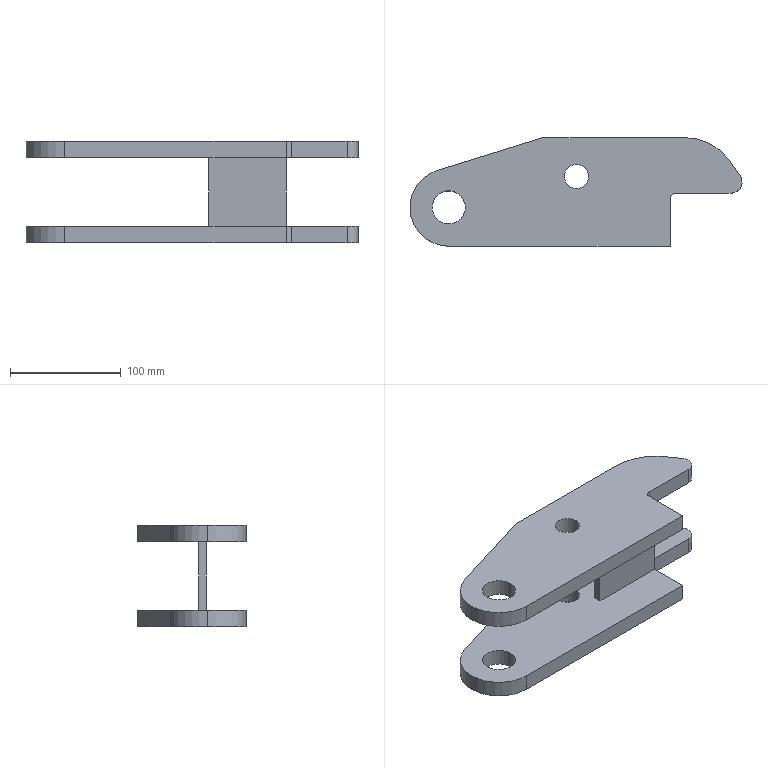Part | SolidWorks | features ICE 2, Extrusion 1, Fillet 1, LPattern 1 | 1 solid | 36 faces | box 300 x 98 x 92 mm | volume 689780 mm3 | cylinder 18 | plane 18 | commonest cylinder face diameters 22 x4 30 x4 70 x4 10 x2 20 x2 100 x2
STEP:
#1=CARTESIAN_POINT('',(-91.605,144.,-1575.828));
#2=VERTEX_POINT('',#1);
#3=CARTESIAN_POINT('',(-69.605,144.,-1575.828));
#4=VERTEX_POINT('',#3);
#5=CARTESIAN_POINT('',(-80.605,144.,-1575.828));
#6=DIRECTION('',(0.,0.,1.));
#7=DIRECTION('',(1.,0.,0.));
#8=AXIS2_PLACEMENT_3D('',#5,#6,#7);
#9=CIRCLE('',#8,11.);
#10=EDGE_CURVE('',#2,#4,#9,.T.);
#11=ORIENTED_EDGE('',*,*,#10,.T.);
#12=CARTESIAN_POINT('',(-69.605,144.,-1590.828));
#13=VERTEX_POINT('',#12);
#14=CARTESIAN_POINT('',(-69.605,144.,-1408.828));
#15=DIRECTION('',(0.,0.,-1.));
#16=VECTOR('',#15,1000.);
#17=LINE('',#14,#16);
#18=EDGE_CURVE('',#4,#13,#17,.T.);
#19=ORIENTED_EDGE('',*,*,#18,.T.);
#20=CARTESIAN_POINT('',(-91.605,144.,-1590.828));
#21=VERTEX_POINT('',#20);
#22=CARTESIAN_POINT('',(-80.605,144.,-1590.828));
#23=DIRECTION('',(0.,0.,1.));
#24=DIRECTION('',(1.,0.,0.));
#25=AXIS2_PLACEMENT_3D('',#22,#23,#24);
#26=CIRCLE('',#25,11.);
#27=EDGE_CURVE('',#21,#13,#26,.T.);
#28=ORIENTED_EDGE('',*,*,#27,.F.);
#29=CARTESIAN_POINT('',(-91.605,144.,-1408.828));
#30=DIRECTION('',(0.,0.,-1.));
#31=VECTOR('',#30,1000.);
#32=LINE('',#29,#31);
#33=EDGE_CURVE('',#2,#21,#32,.T.);
#34=ORIENTED_EDGE('',*,*,#33,.F.);
#35=EDGE_LOOP('',(#11,#19,#28,#34));
#36=FACE_OUTER_BOUND('',#35,.T.);
#37=CARTESIAN_POINT('',(-80.605,144.,-1408.828));
#38=DIRECTION('',(0.,0.,-1.));
#39=DIRECTION('',(-1.,0.,0.));
#40=AXIS2_PLACEMENT_3D('',#37,#38,#39);
#41=CYLINDRICAL_SURFACE('',#40,11.);
#42=ADVANCED_FACE('',(#36),#41,.F.);
#43=CARTESIAN_POINT('',(-91.605,144.,-1498.828));
#44=VERTEX_POINT('',#43);
#45=CARTESIAN_POINT('',(-69.605,144.,-1498.828));
#46=VERTEX_POINT('',#45);
#47=CARTESIAN_POINT('',(-80.605,144.,-1498.828));
#48=DIRECTION('',(0.,0.,1.));
#49=DIRECTION('',(1.,0.,0.));
#50=AXIS2_PLACEMENT_3D('',#47,#48,#49);
#51=CIRCLE('',#50,11.);
#52=EDGE_CURVE('',#44,#46,#51,.T.);
#53=ORIENTED_EDGE('',*,*,#52,.T.);
#54=CARTESIAN_POINT('',(-69.605,144.,-1513.828));
#55=VERTEX_POINT('',#54);
#56=CARTESIAN_POINT('',(-69.605,144.,-1408.828));
#57=DIRECTION('',(0.,0.,-1.));
#58=VECTOR('',#57,1000.);
#59=LINE('',#56,#58);
#60=EDGE_CURVE('',#46,#55,#59,.T.);
#61=ORIENTED_EDGE('',*,*,#60,.T.);
#62=CARTESIAN_POINT('',(-91.605,144.,-1513.828));
#63=VERTEX_POINT('',#62);
#64=CARTESIAN_POINT('',(-80.605,144.,-1513.828));
#65=DIRECTION('',(0.,0.,1.));
#66=DIRECTION('',(1.,0.,0.));
#67=AXIS2_PLACEMENT_3D('',#64,#65,#66);
#68=CIRCLE('',#67,11.);
#69=EDGE_CURVE('',#63,#55,#68,.T.);
#70=ORIENTED_EDGE('',*,*,#69,.F.);
#71=CARTESIAN_POINT('',(-91.605,144.,-1408.828));
#72=DIRECTION('',(0.,0.,-1.));
#73=VECTOR('',#72,1000.);
#74=LINE('',#71,#73);
#75=EDGE_CURVE('',#44,#63,#74,.T.);
#76=ORIENTED_EDGE('',*,*,#75,.F.);
#77=EDGE_LOOP('',(#53,#61,#70,#76));
#78=FACE_OUTER_BOUND('',#77,.T.);
#79=CARTESIAN_POINT('',(-80.605,144.,-1408.828));
#80=DIRECTION('',(0.,0.,-1.));
#81=DIRECTION('',(-1.,0.,0.));
#82=AXIS2_PLACEMENT_3D('',#79,#80,#81);
#83=CYLINDRICAL_SURFACE('',#82,11.);
#84=ADVANCED_FACE('',(#78),#83,.F.);
#85=CARTESIAN_POINT('',(-211.,116.,-1498.828));
#86=VERTEX_POINT('',#85);
#87=CARTESIAN_POINT('',(-181.,116.,-1498.828));
#88=VERTEX_POINT('',#87);
#89=CARTESIAN_POINT('',(-196.,116.,-1498.828));
#90=DIRECTION('',(0.,0.,1.));
#91=DIRECTION('',(1.,0.,0.));
#92=AXIS2_PLACEMENT_3D('',#89,#90,#91);
#93=CIRCLE('',#92,15.);
#94=EDGE_CURVE('',#86,#88,#93,.T.);
#95=ORIENTED_EDGE('',*,*,#94,.T.);
#96=CARTESIAN_POINT('',(-181.,116.,-1513.828));
#97=VERTEX_POINT('',#96);
#98=CARTESIAN_POINT('',(-181.,116.,-1498.828));
#99=DIRECTION('',(0.,0.,-1.));
#100=VECTOR('',#99,1000.);
#101=LINE('',#98,#100);
#102=EDGE_CURVE('',#88,#97,#101,.T.);
#103=ORIENTED_EDGE('',*,*,#102,.T.);
#104=CARTESIAN_POINT('',(-211.,116.,-1513.828));
#105=VERTEX_POINT('',#104);
#106=CARTESIAN_POINT('',(-196.,116.,-1513.828));
#107=DIRECTION('',(0.,0.,1.));
#108=DIRECTION('',(1.,0.,0.));
#109=AXIS2_PLACEMENT_3D('',#106,#107,#108);
#110=CIRCLE('',#109,15.);
#111=EDGE_CURVE('',#105,#97,#110,.T.);
#112=ORIENTED_EDGE('',*,*,#111,.F.);
#113=CARTESIAN_POINT('',(-211.,116.,-1498.828));
#114=DIRECTION('',(0.,0.,-1.));
#115=VECTOR('',#114,1000.);
#116=LINE('',#113,#115);
#117=EDGE_CURVE('',#86,#105,#116,.T.);
#118=ORIENTED_EDGE('',*,*,#117,.F.);
#119=EDGE_LOOP('',(#95,#103,#112,#118));
#120=FACE_OUTER_BOUND('',#119,.T.);
#121=CARTESIAN_POINT('',(-196.,116.,-1498.828));
#122=DIRECTION('',(0.,0.,-1.));
#123=DIRECTION('',(-1.,0.,0.));
#124=AXIS2_PLACEMENT_3D('',#121,#122,#123);
#125=CYLINDRICAL_SURFACE('',#124,15.);
#126=ADVANCED_FACE('',(#120),#125,.F.);
#127=CARTESIAN_POINT('',(-231.,116.,-1498.828));
#128=VERTEX_POINT('',#127);
#129=CARTESIAN_POINT('',(-196.,81.,-1498.828));
#130=VERTEX_POINT('',#129);
#131=CARTESIAN_POINT('',(-196.,116.,-1498.828));
#132=DIRECTION('',(0.,0.,1.));
#133=DIRECTION('',(1.,0.,0.));
#134=AXIS2_PLACEMENT_3D('',#131,#132,#133);
#135=CIRCLE('',#134,35.);
#136=EDGE_CURVE('',#128,#130,#135,.T.);
#137=ORIENTED_EDGE('',*,*,#136,.F.);
#138=CARTESIAN_POINT('',(-231.,116.,-1513.828));
#139=VERTEX_POINT('',#138);
#140=CARTESIAN_POINT('',(-231.,116.,-1498.828));
#141=DIRECTION('',(0.,0.,-1.));
#142=VECTOR('',#141,1000.);
#143=LINE('',#140,#142);
#144=EDGE_CURVE('',#128,#139,#143,.T.);
#145=ORIENTED_EDGE('',*,*,#144,.T.);
#146=CARTESIAN_POINT('',(-196.,81.,-1513.828));
#147=VERTEX_POINT('',#146);
#148=CARTESIAN_POINT('',(-196.,116.,-1513.828));
#149=DIRECTION('',(0.,0.,1.));
#150=DIRECTION('',(1.,0.,0.));
#151=AXIS2_PLACEMENT_3D('',#148,#149,#150);
#152=CIRCLE('',#151,35.);
#153=EDGE_CURVE('',#139,#147,#152,.T.);
#154=ORIENTED_EDGE('',*,*,#153,.T.);
#155=CARTESIAN_POINT('',(-196.,81.,-1498.828));
#156=DIRECTION('',(0.,0.,-1.));
#157=VECTOR('',#156,1000.);
#158=LINE('',#155,#157);
#159=EDGE_CURVE('',#130,#147,#158,.T.);
#160=ORIENTED_EDGE('',*,*,#159,.F.);
#161=EDGE_LOOP('',(#137,#145,#154,#160));
#162=FACE_OUTER_BOUND('',#161,.T.);
#163=CARTESIAN_POINT('',(-196.,116.,-1498.828));
#164=DIRECTION('',(0.,0.,-1.));
#165=DIRECTION('',(-1.,0.,0.));
#166=AXIS2_PLACEMENT_3D('',#163,#164,#165);
#167=CYLINDRICAL_SURFACE('',#166,35.);
#168=ADVANCED_FACE('',(#162),#167,.T.);
#169=CARTESIAN_POINT('',(-211.,116.,-1575.828));
#170=VERTEX_POINT('',#169);
#171=CARTESIAN_POINT('',(-181.,116.,-1575.828));
#172=VERTEX_POINT('',#171);
#173=CARTESIAN_POINT('',(-196.,116.,-1575.828));
#174=DIRECTION('',(0.,0.,1.));
#175=DIRECTION('',(1.,0.,0.));
#176=AXIS2_PLACEMENT_3D('',#173,#174,#175);
#177=CIRCLE('',#176,15.);
#178=EDGE_CURVE('',#170,#172,#177,.T.);
#179=ORIENTED_EDGE('',*,*,#178,.T.);
#180=CARTESIAN_POINT('',(-181.,116.,-1590.828));
#181=VERTEX_POINT('',#180);
#182=CARTESIAN_POINT('',(-181.,116.,-1575.828));
#183=DIRECTION('',(0.,0.,-1.));
#184=VECTOR('',#183,1000.);
#185=LINE('',#182,#184);
#186=EDGE_CURVE('',#172,#181,#185,.T.);
#187=ORIENTED_EDGE('',*,*,#186,.T.);
#188=CARTESIAN_POINT('',(-211.,116.,-1590.828));
#189=VERTEX_POINT('',#188);
#190=CARTESIAN_POINT('',(-196.,116.,-1590.828));
#191=DIRECTION('',(0.,0.,1.));
#192=DIRECTION('',(1.,0.,0.));
#193=AXIS2_PLACEMENT_3D('',#190,#191,#192);
#194=CIRCLE('',#193,15.);
#195=EDGE_CURVE('',#189,#181,#194,.T.);
#196=ORIENTED_EDGE('',*,*,#195,.F.);
#197=CARTESIAN_POINT('',(-211.,116.,-1575.828));
#198=DIRECTION('',(0.,0.,-1.));
#199=VECTOR('',#198,1000.);
#200=LINE('',#197,#199);
#201=EDGE_CURVE('',#170,#189,#200,.T.);
#202=ORIENTED_EDGE('',*,*,#201,.F.);
#203=EDGE_LOOP('',(#179,#187,#196,#202));
#204=FACE_OUTER_BOUND('',#203,.T.);
#205=CARTESIAN_POINT('',(-196.,116.,-1575.828));
#206=DIRECTION('',(0.,0.,-1.));
#207=DIRECTION('',(-1.,0.,0.));
#208=AXIS2_PLACEMENT_3D('',#205,#206,#207);
#209=CYLINDRICAL_SURFACE('',#208,15.);
#210=ADVANCED_FACE('',(#204),#209,.F.);
#211=CARTESIAN_POINT('',(-231.,116.,-1575.828));
#212=VERTEX_POINT('',#211);
#213=CARTESIAN_POINT('',(-196.,81.,-1575.828));
#214=VERTEX_POINT('',#213);
#215=CARTESIAN_POINT('',(-196.,116.,-1575.828));
#216=DIRECTION('',(0.,0.,1.));
#217=DIRECTION('',(1.,0.,0.));
#218=AXIS2_PLACEMENT_3D('',#215,#216,#217);
#219=CIRCLE('',#218,35.);
#220=EDGE_CURVE('',#212,#214,#219,.T.);
#221=ORIENTED_EDGE('',*,*,#220,.F.);
#222=CARTESIAN_POINT('',(-231.,116.,-1590.828));
#223=VERTEX_POINT('',#222);
#224=CARTESIAN_POINT('',(-231.,116.,-1575.828));
#225=DIRECTION('',(0.,0.,-1.));
#226=VECTOR('',#225,1000.);
#227=LINE('',#224,#226);
#228=EDGE_CURVE('',#212,#223,#227,.T.);
#229=ORIENTED_EDGE('',*,*,#228,.T.);
#230=CARTESIAN_POINT('',(-196.,81.,-1590.828));
#231=VERTEX_POINT('',#230);
#232=CARTESIAN_POINT('',(-196.,116.,-1590.828));
#233=DIRECTION('',(0.,0.,1.));
#234=DIRECTION('',(1.,0.,0.));
#235=AXIS2_PLACEMENT_3D('',#232,#233,#234);
#236=CIRCLE('',#235,35.);
#237=EDGE_CURVE('',#223,#231,#236,.T.);
#238=ORIENTED_EDGE('',*,*,#237,.T.);
#239=CARTESIAN_POINT('',(-196.,81.,-1575.828));
#240=DIRECTION('',(0.,0.,-1.));
#241=VECTOR('',#240,1000.);
#242=LINE('',#239,#241);
#243=EDGE_CURVE('',#214,#231,#242,.T.);
#244=ORIENTED_EDGE('',*,*,#243,.F.);
#245=EDGE_LOOP('',(#221,#229,#238,#244));
#246=FACE_OUTER_BOUND('',#245,.T.);
#247=CARTESIAN_POINT('',(-196.,116.,-1575.828));
#248=DIRECTION('',(0.,0.,-1.));
#249=DIRECTION('',(-1.,0.,0.));
#250=AXIS2_PLACEMENT_3D('',#247,#248,#249);
#251=CYLINDRICAL_SURFACE('',#250,35.);
#252=ADVANCED_FACE('',(#246),#251,.T.);
#253=ORIENTED_EDGE('',*,*,#10,.F.);
#254=CARTESIAN_POINT('',(-80.605,144.,-1575.828));
#255=DIRECTION('',(0.,0.,1.));
#256=DIRECTION('',(1.,0.,0.));
#257=AXIS2_PLACEMENT_3D('',#254,#255,#256);
#258=CIRCLE('',#257,11.);
#259=EDGE_CURVE('',#4,#2,#258,.T.);
#260=ORIENTED_EDGE('',*,*,#259,.F.);
#261=EDGE_LOOP('',(#253,#260));
#262=FACE_BOUND('',#261,.T.);
#263=CARTESIAN_POINT('',(-66.,117.,-1575.828));
#264=VERTEX_POINT('',#263);
#265=CARTESIAN_POINT('',(4.,117.,-1575.828));
#266=VERTEX_POINT('',#265);
#267=CARTESIAN_POINT('',(-66.,117.,-1575.828));
#268=DIRECTION('',(1.,0.,0.));
#269=VECTOR('',#268,1000.);
#270=LINE('',#267,#269);
#271=EDGE_CURVE('',#264,#266,#270,.T.);
#272=ORIENTED_EDGE('',*,*,#271,.F.);
#273=CARTESIAN_POINT('',(-66.,124.,-1575.828));
#274=VERTEX_POINT('',#273);
#275=CARTESIAN_POINT('',(-66.,124.,-1575.828));
#276=DIRECTION('',(0.,-1.,0.));
#277=VECTOR('',#276,1000.);
#278=LINE('',#275,#277);
#279=EDGE_CURVE('',#274,#264,#278,.T.);
#280=ORIENTED_EDGE('',*,*,#279,.F.);
#281=CARTESIAN_POINT('',(4.,124.,-1575.828));
#282=VERTEX_POINT('',#281);
#283=CARTESIAN_POINT('',(-66.,124.,-1575.828));
#284=DIRECTION('',(1.,0.,0.));
#285=VECTOR('',#284,1000.);
#286=LINE('',#283,#285);
#287=EDGE_CURVE('',#274,#282,#286,.T.);
#288=ORIENTED_EDGE('',*,*,#287,.T.);
#289=CARTESIAN_POINT('',(9.,129.,-1575.828));
#290=VERTEX_POINT('',#289);
#291=CARTESIAN_POINT('',(9.,124.,-1575.828));
#292=DIRECTION('',(0.,0.,-1.));
#293=DIRECTION('',(1.,0.,0.));
#294=AXIS2_PLACEMENT_3D('',#291,#292,#293);
#295=CIRCLE('',#294,5.);
#296=EDGE_CURVE('',#282,#290,#295,.T.);
#297=ORIENTED_EDGE('',*,*,#296,.T.);
#298=CARTESIAN_POINT('',(59.,129.,-1575.828));
#299=VERTEX_POINT('',#298);
#300=CARTESIAN_POINT('',(59.,129.,-1575.828));
#301=DIRECTION('',(1.,0.,0.));
#302=VECTOR('',#301,1000.);
#303=LINE('',#300,#302);
#304=EDGE_CURVE('',#290,#299,#303,.T.);
#305=ORIENTED_EDGE('',*,*,#304,.T.);
#306=CARTESIAN_POINT('',(67.203,144.719,-1575.828));
#307=VERTEX_POINT('',#306);
#308=CARTESIAN_POINT('',(59.,139.,-1575.828));
#309=DIRECTION('',(0.,0.,1.));
#310=DIRECTION('',(1.,0.,0.));
#311=AXIS2_PLACEMENT_3D('',#308,#309,#310);
#312=CIRCLE('',#311,10.);
#313=EDGE_CURVE('',#299,#307,#312,.T.);
#314=ORIENTED_EDGE('',*,*,#313,.T.);
#315=CARTESIAN_POINT('',(58.224,157.597,-1575.828));
#316=VERTEX_POINT('',#315);
#317=CARTESIAN_POINT('',(58.224,157.597,-1575.828));
#318=DIRECTION('',(-0.5719,0.8203,0.));
#319=VECTOR('',#318,1000.);
#320=LINE('',#317,#319);
#321=EDGE_CURVE('',#307,#316,#320,.T.);
#322=ORIENTED_EDGE('',*,*,#321,.T.);
#323=CARTESIAN_POINT('',(17.209,179.,-1575.828));
#324=VERTEX_POINT('',#323);
#325=CARTESIAN_POINT('',(17.209,129.,-1575.828));
#326=DIRECTION('',(0.,0.,1.));
#327=DIRECTION('',(-1.,0.,0.));
#328=AXIS2_PLACEMENT_3D('',#325,#326,#327);
#329=CIRCLE('',#328,50.);
#330=EDGE_CURVE('',#316,#324,#329,.T.);
#331=ORIENTED_EDGE('',*,*,#330,.T.);
#332=CARTESIAN_POINT('',(-111.,179.,-1575.828));
#333=VERTEX_POINT('',#332);
#334=CARTESIAN_POINT('',(17.209,179.,-1575.828));
#335=DIRECTION('',(-1.,0.,0.));
#336=VECTOR('',#335,1000.);
#337=LINE('',#334,#336);
#338=EDGE_CURVE('',#324,#333,#337,.T.);
#339=ORIENTED_EDGE('',*,*,#338,.T.);
#340=CARTESIAN_POINT('',(-206.366,149.43,-1575.828));
#341=VERTEX_POINT('',#340);
#342=CARTESIAN_POINT('',(-111.,179.,-1575.828));
#343=DIRECTION('',(-0.9551,-0.2962,0.));
#344=VECTOR('',#343,1000.);
#345=LINE('',#342,#344);
#346=EDGE_CURVE('',#333,#341,#345,.T.);
#347=ORIENTED_EDGE('',*,*,#346,.T.);
#348=CARTESIAN_POINT('',(-196.,116.,-1575.828));
#349=DIRECTION('',(0.,0.,1.));
#350=DIRECTION('',(1.,0.,0.));
#351=AXIS2_PLACEMENT_3D('',#348,#349,#350);
#352=CIRCLE('',#351,35.);
#353=EDGE_CURVE('',#341,#212,#352,.T.);
#354=ORIENTED_EDGE('',*,*,#353,.T.);
#355=ORIENTED_EDGE('',*,*,#220,.T.);
#356=CARTESIAN_POINT('',(4.,81.,-1575.828));
#357=VERTEX_POINT('',#356);
#358=CARTESIAN_POINT('',(4.,81.,-1575.828));
#359=DIRECTION('',(1.,0.,0.));
#360=VECTOR('',#359,1000.);
#361=LINE('',#358,#360);
#362=EDGE_CURVE('',#214,#357,#361,.T.);
#363=ORIENTED_EDGE('',*,*,#362,.T.);
#364=CARTESIAN_POINT('',(4.,129.,-1575.828));
#365=DIRECTION('',(0.,1.,0.));
#366=VECTOR('',#365,1000.);
#367=LINE('',#364,#366);
#368=EDGE_CURVE('',#357,#266,#367,.T.);
#369=ORIENTED_EDGE('',*,*,#368,.T.);
#370=EDGE_LOOP('',(#272,#280,#288,#297,#305,#314,#322,#331,#339,#347,#354,#355,#363,#369));
#371=FACE_OUTER_BOUND('',#370,.T.);
#372=ORIENTED_EDGE('',*,*,#178,.F.);
#373=CARTESIAN_POINT('',(-196.,116.,-1575.828));
#374=DIRECTION('',(0.,0.,1.));
#375=DIRECTION('',(1.,0.,0.));
#376=AXIS2_PLACEMENT_3D('',#373,#374,#375);
#377=CIRCLE('',#376,15.);
#378=EDGE_CURVE('',#172,#170,#377,.T.);
#379=ORIENTED_EDGE('',*,*,#378,.F.);
#380=EDGE_LOOP('',(#372,#379));
#381=FACE_BOUND('',#380,.T.);
#382=CARTESIAN_POINT('',(-196.,116.,-1575.828));
#383=DIRECTION('',(0.,0.,1.));
#384=DIRECTION('',(1.,0.,0.));
#385=AXIS2_PLACEMENT_3D('',#382,#383,#384);
#386=PLANE('',#385);
#387=ADVANCED_FACE('',(#262,#371,#381),#386,.T.);
#388=ORIENTED_EDGE('',*,*,#27,.T.);
#389=CARTESIAN_POINT('',(-80.605,144.,-1590.828));
#390=DIRECTION('',(0.,0.,1.));
#391=DIRECTION('',(1.,0.,0.));
#392=AXIS2_PLACEMENT_3D('',#389,#390,#391);
#393=CIRCLE('',#392,11.);
#394=EDGE_CURVE('',#13,#21,#393,.T.);
#395=ORIENTED_EDGE('',*,*,#394,.T.);
#396=EDGE_LOOP('',(#388,#395));
#397=FACE_BOUND('',#396,.T.);
#398=CARTESIAN_POINT('',(4.,81.,-1590.828));
#399=VERTEX_POINT('',#398);
#400=CARTESIAN_POINT('',(4.,124.,-1590.828));
#401=VERTEX_POINT('',#400);
#402=CARTESIAN_POINT('',(4.,129.,-1590.828));
#403=DIRECTION('',(0.,1.,0.));
#404=VECTOR('',#403,1000.);
#405=LINE('',#402,#404);
#406=EDGE_CURVE('',#399,#401,#405,.T.);
#407=ORIENTED_EDGE('',*,*,#406,.F.);
#408=CARTESIAN_POINT('',(4.,81.,-1590.828));
#409=DIRECTION('',(1.,0.,0.));
#410=VECTOR('',#409,1000.);
#411=LINE('',#408,#410);
#412=EDGE_CURVE('',#231,#399,#411,.T.);
#413=ORIENTED_EDGE('',*,*,#412,.F.);
#414=ORIENTED_EDGE('',*,*,#237,.F.);
#415=CARTESIAN_POINT('',(-206.366,149.43,-1590.828));
#416=VERTEX_POINT('',#415);
#417=CARTESIAN_POINT('',(-196.,116.,-1590.828));
#418=DIRECTION('',(0.,0.,1.));
#419=DIRECTION('',(1.,0.,0.));
#420=AXIS2_PLACEMENT_3D('',#417,#418,#419);
#421=CIRCLE('',#420,35.);
#422=EDGE_CURVE('',#416,#223,#421,.T.);
#423=ORIENTED_EDGE('',*,*,#422,.F.);
#424=CARTESIAN_POINT('',(-111.,179.,-1590.828));
#425=VERTEX_POINT('',#424);
#426=CARTESIAN_POINT('',(-111.,179.,-1590.828));
#427=DIRECTION('',(-0.9551,-0.2962,0.));
#428=VECTOR('',#427,1000.);
#429=LINE('',#426,#428);
#430=EDGE_CURVE('',#425,#416,#429,.T.);
#431=ORIENTED_EDGE('',*,*,#430,.F.);
#432=CARTESIAN_POINT('',(17.209,179.,-1590.828));
#433=VERTEX_POINT('',#432);
#434=CARTESIAN_POINT('',(17.209,179.,-1590.828));
#435=DIRECTION('',(-1.,0.,0.));
#436=VECTOR('',#435,1000.);
#437=LINE('',#434,#436);
#438=EDGE_CURVE('',#433,#425,#437,.T.);
#439=ORIENTED_EDGE('',*,*,#438,.F.);
#440=CARTESIAN_POINT('',(58.224,157.597,-1590.828));
#441=VERTEX_POINT('',#440);
#442=CARTESIAN_POINT('',(17.209,129.,-1590.828));
#443=DIRECTION('',(0.,0.,1.));
#444=DIRECTION('',(-1.,0.,0.));
#445=AXIS2_PLACEMENT_3D('',#442,#443,#444);
#446=CIRCLE('',#445,50.);
#447=EDGE_CURVE('',#441,#433,#446,.T.);
#448=ORIENTED_EDGE('',*,*,#447,.F.);
#449=CARTESIAN_POINT('',(67.203,144.719,-1590.828));
#450=VERTEX_POINT('',#449);
#451=CARTESIAN_POINT('',(58.224,157.597,-1590.828));
#452=DIRECTION('',(-0.5719,0.8203,0.));
#453=VECTOR('',#452,1000.);
#454=LINE('',#451,#453);
#455=EDGE_CURVE('',#450,#441,#454,.T.);
#456=ORIENTED_EDGE('',*,*,#455,.F.);
#457=CARTESIAN_POINT('',(59.,129.,-1590.828));
#458=VERTEX_POINT('',#457);
#459=CARTESIAN_POINT('',(59.,139.,-1590.828));
#460=DIRECTION('',(0.,0.,1.));
#461=DIRECTION('',(1.,0.,0.));
#462=AXIS2_PLACEMENT_3D('',#459,#460,#461);
#463=CIRCLE('',#462,10.);
#464=EDGE_CURVE('',#458,#450,#463,.T.);
#465=ORIENTED_EDGE('',*,*,#464,.F.);
#466=CARTESIAN_POINT('',(9.,129.,-1590.828));
#467=VERTEX_POINT('',#466);
#468=CARTESIAN_POINT('',(59.,129.,-1590.828));
#469=DIRECTION('',(1.,0.,0.));
#470=VECTOR('',#469,1000.);
#471=LINE('',#468,#470);
#472=EDGE_CURVE('',#467,#458,#471,.T.);
#473=ORIENTED_EDGE('',*,*,#472,.F.);
#474=CARTESIAN_POINT('',(9.,124.,-1590.828));
#475=DIRECTION('',(0.,0.,1.));
#476=DIRECTION('',(1.,0.,0.));
#477=AXIS2_PLACEMENT_3D('',#474,#475,#476);
#478=CIRCLE('',#477,5.);
#479=EDGE_CURVE('',#467,#401,#478,.T.);
#480=ORIENTED_EDGE('',*,*,#479,.T.);
#481=EDGE_LOOP('',(#407,#413,#414,#423,#431,#439,#448,#456,#465,#473,#480));
#482=FACE_OUTER_BOUND('',#481,.T.);
#483=ORIENTED_EDGE('',*,*,#195,.T.);
#484=CARTESIAN_POINT('',(-196.,116.,-1590.828));
#485=DIRECTION('',(0.,0.,1.));
#486=DIRECTION('',(1.,0.,0.));
#487=AXIS2_PLACEMENT_3D('',#484,#485,#486);
#488=CIRCLE('',#487,15.);
#489=EDGE_CURVE('',#181,#189,#488,.T.);
#490=ORIENTED_EDGE('',*,*,#489,.T.);
#491=EDGE_LOOP('',(#483,#490));
#492=FACE_BOUND('',#491,.T.);
#493=CARTESIAN_POINT('',(-196.,116.,-1590.828));
#494=DIRECTION('',(0.,0.,1.));
#495=DIRECTION('',(1.,0.,0.));
#496=AXIS2_PLACEMENT_3D('',#493,#494,#495);
#497=PLANE('',#496);
#498=ADVANCED_FACE('',(#397,#482,#492),#497,.F.);
#499=ORIENTED_EDGE('',*,*,#406,.T.);
#500=CARTESIAN_POINT('',(4.,124.,-1575.828));
#501=DIRECTION('',(0.,0.,1.));
#502=VECTOR('',#501,1000.);
#503=LINE('',#500,#502);
#504=EDGE_CURVE('',#401,#282,#503,.T.);
#505=ORIENTED_EDGE('',*,*,#504,.T.);
#506=CARTESIAN_POINT('',(4.,124.,-1513.828));
#507=VERTEX_POINT('',#506);
#508=CARTESIAN_POINT('',(4.,124.,-1575.828));
#509=DIRECTION('',(0.,0.,-1.));
#510=VECTOR('',#509,1000.);
#511=LINE('',#508,#510);
#512=EDGE_CURVE('',#507,#282,#511,.T.);
#513=ORIENTED_EDGE('',*,*,#512,.F.);
#514=CARTESIAN_POINT('',(4.,124.,-1498.828));
#515=VERTEX_POINT('',#514);
#516=CARTESIAN_POINT('',(4.,124.,-1498.828));
#517=DIRECTION('',(0.,0.,1.));
#518=VECTOR('',#517,1000.);
#519=LINE('',#516,#518);
#520=EDGE_CURVE('',#507,#515,#519,.T.);
#521=ORIENTED_EDGE('',*,*,#520,.T.);
#522=CARTESIAN_POINT('',(4.,81.,-1498.828));
#523=VERTEX_POINT('',#522);
#524=CARTESIAN_POINT('',(4.,129.,-1498.828));
#525=DIRECTION('',(0.,1.,0.));
#526=VECTOR('',#525,1000.);
#527=LINE('',#524,#526);
#528=EDGE_CURVE('',#523,#515,#527,.T.);
#529=ORIENTED_EDGE('',*,*,#528,.F.);
#530=CARTESIAN_POINT('',(4.,81.,-1513.828));
#531=VERTEX_POINT('',#530);
#532=CARTESIAN_POINT('',(4.,81.,-1498.828));
#533=DIRECTION('',(0.,0.,-1.));
#534=VECTOR('',#533,1000.);
#535=LINE('',#532,#534);
#536=EDGE_CURVE('',#523,#531,#535,.T.);
#537=ORIENTED_EDGE('',*,*,#536,.T.);
#538=CARTESIAN_POINT('',(4.,117.,-1513.828));
#539=VERTEX_POINT('',#538);
#540=CARTESIAN_POINT('',(4.,129.,-1513.828));
#541=DIRECTION('',(0.,1.,0.));
#542=VECTOR('',#541,1000.);
#543=LINE('',#540,#542);
#544=EDGE_CURVE('',#531,#539,#543,.T.);
#545=ORIENTED_EDGE('',*,*,#544,.T.);
#546=CARTESIAN_POINT('',(4.,117.,-1575.828));
#547=DIRECTION('',(0.,0.,1.));
#548=VECTOR('',#547,1000.);
#549=LINE('',#546,#548);
#550=EDGE_CURVE('',#266,#539,#549,.T.);
#551=ORIENTED_EDGE('',*,*,#550,.F.);
#552=ORIENTED_EDGE('',*,*,#368,.F.);
#553=CARTESIAN_POINT('',(4.,81.,-1575.828));
#554=DIRECTION('',(0.,0.,-1.));
#555=VECTOR('',#554,1000.);
#556=LINE('',#553,#555);
#557=EDGE_CURVE('',#357,#399,#556,.T.);
#558=ORIENTED_EDGE('',*,*,#557,.T.);
#559=EDGE_LOOP('',(#499,#505,#513,#521,#529,#537,#545,#551,#552,#558));
#560=FACE_OUTER_BOUND('',#559,.T.);
#561=CARTESIAN_POINT('',(4.,129.,-1575.828));
#562=DIRECTION('',(-1.,0.,0.));
#563=DIRECTION('',(0.,-1.,0.));
#564=AXIS2_PLACEMENT_3D('',#561,#562,#563);
#565=PLANE('',#564);
#566=ADVANCED_FACE('',(#560),#565,.F.);
#567=ORIENTED_EDGE('',*,*,#304,.F.);
#568=CARTESIAN_POINT('',(9.,129.,-1590.828));
#569=DIRECTION('',(0.,0.,-1.));
#570=VECTOR('',#569,1000.);
#571=LINE('',#568,#570);
#572=EDGE_CURVE('',#290,#467,#571,.T.);
#573=ORIENTED_EDGE('',*,*,#572,.T.);
#574=ORIENTED_EDGE('',*,*,#472,.T.);
#575=CARTESIAN_POINT('',(59.,129.,-1575.828));
#576=DIRECTION('',(0.,0.,-1.));
#577=VECTOR('',#576,1000.);
#578=LINE('',#575,#577);
#579=EDGE_CURVE('',#299,#458,#578,.T.);
#580=ORIENTED_EDGE('',*,*,#579,.F.);
#581=EDGE_LOOP('',(#567,#573,#574,#580));
#582=FACE_OUTER_BOUND('',#581,.T.);
#583=CARTESIAN_POINT('',(59.,129.,-1575.828));
#584=DIRECTION('',(0.,1.,0.));
#585=DIRECTION('',(-1.,0.,0.));
#586=AXIS2_PLACEMENT_3D('',#583,#584,#585);
#587=PLANE('',#586);
#588=ADVANCED_FACE('',(#582),#587,.F.);
#589=ORIENTED_EDGE('',*,*,#464,.T.);
#590=CARTESIAN_POINT('',(67.203,144.719,-1575.828));
#591=DIRECTION('',(0.,0.,-1.));
#592=VECTOR('',#591,1000.);
#593=LINE('',#590,#592);
#594=EDGE_CURVE('',#307,#450,#593,.T.);
#595=ORIENTED_EDGE('',*,*,#594,.F.);
#596=ORIENTED_EDGE('',*,*,#313,.F.);
#597=ORIENTED_EDGE('',*,*,#579,.T.);
#598=EDGE_LOOP('',(#589,#595,#596,#597));
#599=FACE_OUTER_BOUND('',#598,.T.);
#600=CARTESIAN_POINT('',(59.,139.,-1575.828));
#601=DIRECTION('',(0.,0.,-1.));
#602=DIRECTION('',(-1.,0.,0.));
#603=AXIS2_PLACEMENT_3D('',#600,#601,#602);
#604=CYLINDRICAL_SURFACE('',#603,10.);
#605=ADVANCED_FACE('',(#599),#604,.T.);
#606=ORIENTED_EDGE('',*,*,#455,.T.);
#607=CARTESIAN_POINT('',(58.224,157.597,-1575.828));
#608=DIRECTION('',(0.,0.,-1.));
#609=VECTOR('',#608,1000.);
#610=LINE('',#607,#609);
#611=EDGE_CURVE('',#316,#441,#610,.T.);
#612=ORIENTED_EDGE('',*,*,#611,.F.);
#613=ORIENTED_EDGE('',*,*,#321,.F.);
#614=ORIENTED_EDGE('',*,*,#594,.T.);
#615=EDGE_LOOP('',(#606,#612,#613,#614));
#616=FACE_OUTER_BOUND('',#615,.T.);
#617=CARTESIAN_POINT('',(58.224,157.597,-1575.828));
#618=DIRECTION('',(-0.8203,-0.5719,0.));
#619=DIRECTION('',(0.5719,-0.8203,0.));
#620=AXIS2_PLACEMENT_3D('',#617,#618,#619);
#621=PLANE('',#620);
#622=ADVANCED_FACE('',(#616),#621,.F.);
#623=ORIENTED_EDGE('',*,*,#447,.T.);
#624=CARTESIAN_POINT('',(17.209,179.,-1575.828));
#625=DIRECTION('',(0.,0.,-1.));
#626=VECTOR('',#625,1000.);
#627=LINE('',#624,#626);
#628=EDGE_CURVE('',#324,#433,#627,.T.);
#629=ORIENTED_EDGE('',*,*,#628,.F.);
#630=ORIENTED_EDGE('',*,*,#330,.F.);
#631=ORIENTED_EDGE('',*,*,#611,.T.);
#632=EDGE_LOOP('',(#623,#629,#630,#631));
#633=FACE_OUTER_BOUND('',#632,.T.);
#634=CARTESIAN_POINT('',(17.209,129.,-1575.828));
#635=DIRECTION('',(0.,0.,-1.));
#636=DIRECTION('',(-1.,0.,0.));
#637=AXIS2_PLACEMENT_3D('',#634,#635,#636);
#638=CYLINDRICAL_SURFACE('',#637,50.);
#639=ADVANCED_FACE('',(#633),#638,.T.);
#640=ORIENTED_EDGE('',*,*,#438,.T.);
#641=CARTESIAN_POINT('',(-111.,179.,-1575.828));
#642=DIRECTION('',(0.,0.,-1.));
#643=VECTOR('',#642,1000.);
#644=LINE('',#641,#643);
#645=EDGE_CURVE('',#333,#425,#644,.T.);
#646=ORIENTED_EDGE('',*,*,#645,.F.);
#647=ORIENTED_EDGE('',*,*,#338,.F.);
#648=ORIENTED_EDGE('',*,*,#628,.T.);
#649=EDGE_LOOP('',(#640,#646,#647,#648));
#650=FACE_OUTER_BOUND('',#649,.T.);
#651=CARTESIAN_POINT('',(17.209,179.,-1575.828));
#652=DIRECTION('',(0.,-1.,0.));
#653=DIRECTION('',(1.,0.,0.));
#654=AXIS2_PLACEMENT_3D('',#651,#652,#653);
#655=PLANE('',#654);
#656=ADVANCED_FACE('',(#650),#655,.F.);
#657=ORIENTED_EDGE('',*,*,#430,.T.);
#658=CARTESIAN_POINT('',(-206.366,149.43,-1575.828));
#659=DIRECTION('',(0.,0.,-1.));
#660=VECTOR('',#659,1000.);
#661=LINE('',#658,#660);
#662=EDGE_CURVE('',#341,#416,#661,.T.);
#663=ORIENTED_EDGE('',*,*,#662,.F.);
#664=ORIENTED_EDGE('',*,*,#346,.F.);
#665=ORIENTED_EDGE('',*,*,#645,.T.);
#666=EDGE_LOOP('',(#657,#663,#664,#665));
#667=FACE_OUTER_BOUND('',#666,.T.);
#668=CARTESIAN_POINT('',(-111.,179.,-1575.828));
#669=DIRECTION('',(0.2962,-0.9551,0.));
#670=DIRECTION('',(0.9551,0.2962,0.));
#671=AXIS2_PLACEMENT_3D('',#668,#669,#670);
#672=PLANE('',#671);
#673=ADVANCED_FACE('',(#667),#672,.F.);
#674=ORIENTED_EDGE('',*,*,#228,.F.);
#675=ORIENTED_EDGE('',*,*,#353,.F.);
#676=ORIENTED_EDGE('',*,*,#662,.T.);
#677=ORIENTED_EDGE('',*,*,#422,.T.);
#678=EDGE_LOOP('',(#674,#675,#676,#677));
#679=FACE_OUTER_BOUND('',#678,.T.);
#680=CARTESIAN_POINT('',(-196.,116.,-1575.828));
#681=DIRECTION('',(0.,0.,-1.));
#682=DIRECTION('',(-1.,0.,0.));
#683=AXIS2_PLACEMENT_3D('',#680,#681,#682);
#684=CYLINDRICAL_SURFACE('',#683,35.);
#685=ADVANCED_FACE('',(#679),#684,.T.);
#686=ORIENTED_EDGE('',*,*,#412,.T.);
#687=ORIENTED_EDGE('',*,*,#557,.F.);
#688=ORIENTED_EDGE('',*,*,#362,.F.);
#689=ORIENTED_EDGE('',*,*,#243,.T.);
#690=EDGE_LOOP('',(#686,#687,#688,#689));
#691=FACE_OUTER_BOUND('',#690,.T.);
#692=CARTESIAN_POINT('',(4.,81.,-1575.828));
#693=DIRECTION('',(0.,1.,0.));
#694=DIRECTION('',(-1.,0.,0.));
#695=AXIS2_PLACEMENT_3D('',#692,#693,#694);
#696=PLANE('',#695);
#697=ADVANCED_FACE('',(#691),#696,.F.);
#698=ORIENTED_EDGE('',*,*,#186,.F.);
#699=ORIENTED_EDGE('',*,*,#378,.T.);
#700=ORIENTED_EDGE('',*,*,#201,.T.);
#701=ORIENTED_EDGE('',*,*,#489,.F.);
#702=EDGE_LOOP('',(#698,#699,#700,#701));
#703=FACE_OUTER_BOUND('',#702,.T.);
#704=CARTESIAN_POINT('',(-196.,116.,-1575.828));
#705=DIRECTION('',(0.,0.,-1.));
#706=DIRECTION('',(-1.,0.,0.));
#707=AXIS2_PLACEMENT_3D('',#704,#705,#706);
#708=CYLINDRICAL_SURFACE('',#707,15.);
#709=ADVANCED_FACE('',(#703),#708,.F.);
#710=ORIENTED_EDGE('',*,*,#550,.T.);
#711=CARTESIAN_POINT('',(-66.,117.,-1513.828));
#712=VERTEX_POINT('',#711);
#713=CARTESIAN_POINT('',(-66.,117.,-1513.828));
#714=DIRECTION('',(1.,0.,0.));
#715=VECTOR('',#714,1000.);
#716=LINE('',#713,#715);
#717=EDGE_CURVE('',#712,#539,#716,.T.);
#718=ORIENTED_EDGE('',*,*,#717,.F.);
#719=CARTESIAN_POINT('',(-66.,117.,-1575.828));
#720=DIRECTION('',(0.,0.,1.));
#721=VECTOR('',#720,1000.);
#722=LINE('',#719,#721);
#723=EDGE_CURVE('',#264,#712,#722,.T.);
#724=ORIENTED_EDGE('',*,*,#723,.F.);
#725=ORIENTED_EDGE('',*,*,#271,.T.);
#726=EDGE_LOOP('',(#710,#718,#724,#725));
#727=FACE_OUTER_BOUND('',#726,.T.);
#728=CARTESIAN_POINT('',(-66.,117.,-1575.828));
#729=DIRECTION('',(0.,1.,0.));
#730=DIRECTION('',(-1.,0.,0.));
#731=AXIS2_PLACEMENT_3D('',#728,#729,#730);
#732=PLANE('',#731);
#733=ADVANCED_FACE('',(#727),#732,.F.);
#734=ORIENTED_EDGE('',*,*,#512,.T.);
#735=ORIENTED_EDGE('',*,*,#287,.F.);
#736=CARTESIAN_POINT('',(-66.,124.,-1513.828));
#737=VERTEX_POINT('',#736);
#738=CARTESIAN_POINT('',(-66.,124.,-1575.828));
#739=DIRECTION('',(0.,0.,-1.));
#740=VECTOR('',#739,1000.);
#741=LINE('',#738,#740);
#742=EDGE_CURVE('',#737,#274,#741,.T.);
#743=ORIENTED_EDGE('',*,*,#742,.F.);
#744=CARTESIAN_POINT('',(-66.,124.,-1513.828));
#745=DIRECTION('',(1.,0.,0.));
#746=VECTOR('',#745,1000.);
#747=LINE('',#744,#746);
#748=EDGE_CURVE('',#737,#507,#747,.T.);
#749=ORIENTED_EDGE('',*,*,#748,.T.);
#750=EDGE_LOOP('',(#734,#735,#743,#749));
#751=FACE_OUTER_BOUND('',#750,.T.);
#752=CARTESIAN_POINT('',(-66.,124.,-1575.828));
#753=DIRECTION('',(0.,-1.,0.));
#754=DIRECTION('',(1.,0.,0.));
#755=AXIS2_PLACEMENT_3D('',#752,#753,#754);
#756=PLANE('',#755);
#757=ADVANCED_FACE('',(#751),#756,.F.);
#758=ORIENTED_EDGE('',*,*,#279,.T.);
#759=ORIENTED_EDGE('',*,*,#723,.T.);
#760=CARTESIAN_POINT('',(-66.,124.,-1513.828));
#761=DIRECTION('',(0.,1.,0.));
#762=VECTOR('',#761,1000.);
#763=LINE('',#760,#762);
#764=EDGE_CURVE('',#712,#737,#763,.T.);
#765=ORIENTED_EDGE('',*,*,#764,.T.);
#766=ORIENTED_EDGE('',*,*,#742,.T.);
#767=EDGE_LOOP('',(#758,#759,#765,#766));
#768=FACE_OUTER_BOUND('',#767,.T.);
#769=CARTESIAN_POINT('',(-66.,117.,-1575.828));
#770=DIRECTION('',(-1.,0.,0.));
#771=DIRECTION('',(0.,-1.,0.));
#772=AXIS2_PLACEMENT_3D('',#769,#770,#771);
#773=PLANE('',#772);
#774=ADVANCED_FACE('',(#768),#773,.T.);
#775=ORIENTED_EDGE('',*,*,#52,.F.);
#776=CARTESIAN_POINT('',(-80.605,144.,-1498.828));
#777=DIRECTION('',(0.,0.,1.));
#778=DIRECTION('',(1.,0.,0.));
#779=AXIS2_PLACEMENT_3D('',#776,#777,#778);
#780=CIRCLE('',#779,11.);
#781=EDGE_CURVE('',#46,#44,#780,.T.);
#782=ORIENTED_EDGE('',*,*,#781,.F.);
#783=EDGE_LOOP('',(#775,#782));
#784=FACE_BOUND('',#783,.T.);
#785=ORIENTED_EDGE('',*,*,#528,.T.);
#786=CARTESIAN_POINT('',(9.,129.,-1498.828));
#787=VERTEX_POINT('',#786);
#788=CARTESIAN_POINT('',(9.,124.,-1498.828));
#789=DIRECTION('',(0.,0.,-1.));
#790=DIRECTION('',(1.,0.,0.));
#791=AXIS2_PLACEMENT_3D('',#788,#789,#790);
#792=CIRCLE('',#791,5.);
#793=EDGE_CURVE('',#515,#787,#792,.T.);
#794=ORIENTED_EDGE('',*,*,#793,.T.);
#795=CARTESIAN_POINT('',(59.,129.,-1498.828));
#796=VERTEX_POINT('',#795);
#797=CARTESIAN_POINT('',(59.,129.,-1498.828));
#798=DIRECTION('',(1.,0.,0.));
#799=VECTOR('',#798,1000.);
#800=LINE('',#797,#799);
#801=EDGE_CURVE('',#787,#796,#800,.T.);
#802=ORIENTED_EDGE('',*,*,#801,.T.);
#803=CARTESIAN_POINT('',(67.203,144.719,-1498.828));
#804=VERTEX_POINT('',#803);
#805=CARTESIAN_POINT('',(59.,139.,-1498.828));
#806=DIRECTION('',(0.,0.,1.));
#807=DIRECTION('',(1.,0.,0.));
#808=AXIS2_PLACEMENT_3D('',#805,#806,#807);
#809=CIRCLE('',#808,10.);
#810=EDGE_CURVE('',#796,#804,#809,.T.);
#811=ORIENTED_EDGE('',*,*,#810,.T.);
#812=CARTESIAN_POINT('',(58.224,157.597,-1498.828));
#813=VERTEX_POINT('',#812);
#814=CARTESIAN_POINT('',(58.224,157.597,-1498.828));
#815=DIRECTION('',(-0.5719,0.8203,0.));
#816=VECTOR('',#815,1000.);
#817=LINE('',#814,#816);
#818=EDGE_CURVE('',#804,#813,#817,.T.);
#819=ORIENTED_EDGE('',*,*,#818,.T.);
#820=CARTESIAN_POINT('',(17.209,179.,-1498.828));
#821=VERTEX_POINT('',#820);
#822=CARTESIAN_POINT('',(17.209,129.,-1498.828));
#823=DIRECTION('',(0.,0.,1.));
#824=DIRECTION('',(-1.,0.,0.));
#825=AXIS2_PLACEMENT_3D('',#822,#823,#824);
#826=CIRCLE('',#825,50.);
#827=EDGE_CURVE('',#813,#821,#826,.T.);
#828=ORIENTED_EDGE('',*,*,#827,.T.);
#829=CARTESIAN_POINT('',(-111.,179.,-1498.828));
#830=VERTEX_POINT('',#829);
#831=CARTESIAN_POINT('',(17.209,179.,-1498.828));
#832=DIRECTION('',(-1.,0.,0.));
#833=VECTOR('',#832,1000.);
#834=LINE('',#831,#833);
#835=EDGE_CURVE('',#821,#830,#834,.T.);
#836=ORIENTED_EDGE('',*,*,#835,.T.);
#837=CARTESIAN_POINT('',(-206.366,149.43,-1498.828));
#838=VERTEX_POINT('',#837);
#839=CARTESIAN_POINT('',(-111.,179.,-1498.828));
#840=DIRECTION('',(-0.9551,-0.2962,0.));
#841=VECTOR('',#840,1000.);
#842=LINE('',#839,#841);
#843=EDGE_CURVE('',#830,#838,#842,.T.);
#844=ORIENTED_EDGE('',*,*,#843,.T.);
#845=CARTESIAN_POINT('',(-196.,116.,-1498.828));
#846=DIRECTION('',(0.,0.,1.));
#847=DIRECTION('',(1.,0.,0.));
#848=AXIS2_PLACEMENT_3D('',#845,#846,#847);
#849=CIRCLE('',#848,35.);
#850=EDGE_CURVE('',#838,#128,#849,.T.);
#851=ORIENTED_EDGE('',*,*,#850,.T.);
#852=ORIENTED_EDGE('',*,*,#136,.T.);
#853=CARTESIAN_POINT('',(4.,81.,-1498.828));
#854=DIRECTION('',(1.,0.,0.));
#855=VECTOR('',#854,1000.);
#856=LINE('',#853,#855);
#857=EDGE_CURVE('',#130,#523,#856,.T.);
#858=ORIENTED_EDGE('',*,*,#857,.T.);
#859=EDGE_LOOP('',(#785,#794,#802,#811,#819,#828,#836,#844,#851,#852,#858));
#860=FACE_OUTER_BOUND('',#859,.T.);
#861=ORIENTED_EDGE('',*,*,#94,.F.);
#862=CARTESIAN_POINT('',(-196.,116.,-1498.828));
#863=DIRECTION('',(0.,0.,1.));
#864=DIRECTION('',(1.,0.,0.));
#865=AXIS2_PLACEMENT_3D('',#862,#863,#864);
#866=CIRCLE('',#865,15.);
#867=EDGE_CURVE('',#88,#86,#866,.T.);
#868=ORIENTED_EDGE('',*,*,#867,.F.);
#869=EDGE_LOOP('',(#861,#868));
#870=FACE_BOUND('',#869,.T.);
#871=CARTESIAN_POINT('',(-196.,116.,-1498.828));
#872=DIRECTION('',(0.,0.,1.));
#873=DIRECTION('',(1.,0.,0.));
#874=AXIS2_PLACEMENT_3D('',#871,#872,#873);
#875=PLANE('',#874);
#876=ADVANCED_FACE('',(#784,#860,#870),#875,.T.);
#877=ORIENTED_EDGE('',*,*,#69,.T.);
#878=CARTESIAN_POINT('',(-80.605,144.,-1513.828));
#879=DIRECTION('',(0.,0.,1.));
#880=DIRECTION('',(1.,0.,0.));
#881=AXIS2_PLACEMENT_3D('',#878,#879,#880);
#882=CIRCLE('',#881,11.);
#883=EDGE_CURVE('',#55,#63,#882,.T.);
#884=ORIENTED_EDGE('',*,*,#883,.T.);
#885=EDGE_LOOP('',(#877,#884));
#886=FACE_BOUND('',#885,.T.);
#887=ORIENTED_EDGE('',*,*,#748,.F.);
#888=ORIENTED_EDGE('',*,*,#764,.F.);
#889=ORIENTED_EDGE('',*,*,#717,.T.);
#890=ORIENTED_EDGE('',*,*,#544,.F.);
#891=CARTESIAN_POINT('',(4.,81.,-1513.828));
#892=DIRECTION('',(1.,0.,0.));
#893=VECTOR('',#892,1000.);
#894=LINE('',#891,#893);
#895=EDGE_CURVE('',#147,#531,#894,.T.);
#896=ORIENTED_EDGE('',*,*,#895,.F.);
#897=ORIENTED_EDGE('',*,*,#153,.F.);
#898=CARTESIAN_POINT('',(-206.366,149.43,-1513.828));
#899=VERTEX_POINT('',#898);
#900=CARTESIAN_POINT('',(-196.,116.,-1513.828));
#901=DIRECTION('',(0.,0.,1.));
#902=DIRECTION('',(1.,0.,0.));
#903=AXIS2_PLACEMENT_3D('',#900,#901,#902);
#904=CIRCLE('',#903,35.);
#905=EDGE_CURVE('',#899,#139,#904,.T.);
#906=ORIENTED_EDGE('',*,*,#905,.F.);
#907=CARTESIAN_POINT('',(-111.,179.,-1513.828));
#908=VERTEX_POINT('',#907);
#909=CARTESIAN_POINT('',(-111.,179.,-1513.828));
#910=DIRECTION('',(-0.9551,-0.2962,0.));
#911=VECTOR('',#910,1000.);
#912=LINE('',#909,#911);
#913=EDGE_CURVE('',#908,#899,#912,.T.);
#914=ORIENTED_EDGE('',*,*,#913,.F.);
#915=CARTESIAN_POINT('',(17.209,179.,-1513.828));
#916=VERTEX_POINT('',#915);
#917=CARTESIAN_POINT('',(17.209,179.,-1513.828));
#918=DIRECTION('',(-1.,0.,0.));
#919=VECTOR('',#918,1000.);
#920=LINE('',#917,#919);
#921=EDGE_CURVE('',#916,#908,#920,.T.);
#922=ORIENTED_EDGE('',*,*,#921,.F.);
#923=CARTESIAN_POINT('',(58.224,157.597,-1513.828));
#924=VERTEX_POINT('',#923);
#925=CARTESIAN_POINT('',(17.209,129.,-1513.828));
#926=DIRECTION('',(0.,0.,1.));
#927=DIRECTION('',(-1.,0.,0.));
#928=AXIS2_PLACEMENT_3D('',#925,#926,#927);
#929=CIRCLE('',#928,50.);
#930=EDGE_CURVE('',#924,#916,#929,.T.);
#931=ORIENTED_EDGE('',*,*,#930,.F.);
#932=CARTESIAN_POINT('',(67.203,144.719,-1513.828));
#933=VERTEX_POINT('',#932);
#934=CARTESIAN_POINT('',(58.224,157.597,-1513.828));
#935=DIRECTION('',(-0.5719,0.8203,0.));
#936=VECTOR('',#935,1000.);
#937=LINE('',#934,#936);
#938=EDGE_CURVE('',#933,#924,#937,.T.);
#939=ORIENTED_EDGE('',*,*,#938,.F.);
#940=CARTESIAN_POINT('',(59.,129.,-1513.828));
#941=VERTEX_POINT('',#940);
#942=CARTESIAN_POINT('',(59.,139.,-1513.828));
#943=DIRECTION('',(0.,0.,1.));
#944=DIRECTION('',(1.,0.,0.));
#945=AXIS2_PLACEMENT_3D('',#942,#943,#944);
#946=CIRCLE('',#945,10.);
#947=EDGE_CURVE('',#941,#933,#946,.T.);
#948=ORIENTED_EDGE('',*,*,#947,.F.);
#949=CARTESIAN_POINT('',(9.,129.,-1513.828));
#950=VERTEX_POINT('',#949);
#951=CARTESIAN_POINT('',(59.,129.,-1513.828));
#952=DIRECTION('',(1.,0.,0.));
#953=VECTOR('',#952,1000.);
#954=LINE('',#951,#953);
#955=EDGE_CURVE('',#950,#941,#954,.T.);
#956=ORIENTED_EDGE('',*,*,#955,.F.);
#957=CARTESIAN_POINT('',(9.,124.,-1513.828));
#958=DIRECTION('',(0.,0.,1.));
#959=DIRECTION('',(1.,0.,0.));
#960=AXIS2_PLACEMENT_3D('',#957,#958,#959);
#961=CIRCLE('',#960,5.);
#962=EDGE_CURVE('',#950,#507,#961,.T.);
#963=ORIENTED_EDGE('',*,*,#962,.T.);
#964=EDGE_LOOP('',(#887,#888,#889,#890,#896,#897,#906,#914,#922,#931,#939,#948,#956,#963));
#965=FACE_OUTER_BOUND('',#964,.T.);
#966=ORIENTED_EDGE('',*,*,#111,.T.);
#967=CARTESIAN_POINT('',(-196.,116.,-1513.828));
#968=DIRECTION('',(0.,0.,1.));
#969=DIRECTION('',(1.,0.,0.));
#970=AXIS2_PLACEMENT_3D('',#967,#968,#969);
#971=CIRCLE('',#970,15.);
#972=EDGE_CURVE('',#97,#105,#971,.T.);
#973=ORIENTED_EDGE('',*,*,#972,.T.);
#974=EDGE_LOOP('',(#966,#973));
#975=FACE_BOUND('',#974,.T.);
#976=CARTESIAN_POINT('',(-196.,116.,-1513.828));
#977=DIRECTION('',(0.,0.,1.));
#978=DIRECTION('',(1.,0.,0.));
#979=AXIS2_PLACEMENT_3D('',#976,#977,#978);
#980=PLANE('',#979);
#981=ADVANCED_FACE('',(#886,#965,#975),#980,.F.);
#982=ORIENTED_EDGE('',*,*,#801,.F.);
#983=CARTESIAN_POINT('',(9.,129.,-1513.828));
#984=DIRECTION('',(0.,0.,-1.));
#985=VECTOR('',#984,1000.);
#986=LINE('',#983,#985);
#987=EDGE_CURVE('',#787,#950,#986,.T.);
#988=ORIENTED_EDGE('',*,*,#987,.T.);
#989=ORIENTED_EDGE('',*,*,#955,.T.);
#990=CARTESIAN_POINT('',(59.,129.,-1498.828));
#991=DIRECTION('',(0.,0.,-1.));
#992=VECTOR('',#991,1000.);
#993=LINE('',#990,#992);
#994=EDGE_CURVE('',#796,#941,#993,.T.);
#995=ORIENTED_EDGE('',*,*,#994,.F.);
#996=EDGE_LOOP('',(#982,#988,#989,#995));
#997=FACE_OUTER_BOUND('',#996,.T.);
#998=CARTESIAN_POINT('',(59.,129.,-1498.828));
#999=DIRECTION('',(0.,1.,0.));
#1000=DIRECTION('',(-1.,0.,0.));
#1001=AXIS2_PLACEMENT_3D('',#998,#999,#1000);
#1002=PLANE('',#1001);
#1003=ADVANCED_FACE('',(#997),#1002,.F.);
#1004=ORIENTED_EDGE('',*,*,#947,.T.);
#1005=CARTESIAN_POINT('',(67.203,144.719,-1498.828));
#1006=DIRECTION('',(0.,0.,-1.));
#1007=VECTOR('',#1006,1000.);
#1008=LINE('',#1005,#1007);
#1009=EDGE_CURVE('',#804,#933,#1008,.T.);
#1010=ORIENTED_EDGE('',*,*,#1009,.F.);
#1011=ORIENTED_EDGE('',*,*,#810,.F.);
#1012=ORIENTED_EDGE('',*,*,#994,.T.);
#1013=EDGE_LOOP('',(#1004,#1010,#1011,#1012));
#1014=FACE_OUTER_BOUND('',#1013,.T.);
#1015=CARTESIAN_POINT('',(59.,139.,-1498.828));
#1016=DIRECTION('',(0.,0.,-1.));
#1017=DIRECTION('',(-1.,0.,0.));
#1018=AXIS2_PLACEMENT_3D('',#1015,#1016,#1017);
#1019=CYLINDRICAL_SURFACE('',#1018,10.);
#1020=ADVANCED_FACE('',(#1014),#1019,.T.);
#1021=ORIENTED_EDGE('',*,*,#938,.T.);
#1022=CARTESIAN_POINT('',(58.224,157.597,-1498.828));
#1023=DIRECTION('',(0.,0.,-1.));
#1024=VECTOR('',#1023,1000.);
#1025=LINE('',#1022,#1024);
#1026=EDGE_CURVE('',#813,#924,#1025,.T.);
#1027=ORIENTED_EDGE('',*,*,#1026,.F.);
#1028=ORIENTED_EDGE('',*,*,#818,.F.);
#1029=ORIENTED_EDGE('',*,*,#1009,.T.);
#1030=EDGE_LOOP('',(#1021,#1027,#1028,#1029));
#1031=FACE_OUTER_BOUND('',#1030,.T.);
#1032=CARTESIAN_POINT('',(58.224,157.597,-1498.828));
#1033=DIRECTION('',(-0.8203,-0.5719,0.));
#1034=DIRECTION('',(0.5719,-0.8203,0.));
#1035=AXIS2_PLACEMENT_3D('',#1032,#1033,#1034);
#1036=PLANE('',#1035);
#1037=ADVANCED_FACE('',(#1031),#1036,.F.);
#1038=ORIENTED_EDGE('',*,*,#930,.T.);
#1039=CARTESIAN_POINT('',(17.209,179.,-1498.828));
#1040=DIRECTION('',(0.,0.,-1.));
#1041=VECTOR('',#1040,1000.);
#1042=LINE('',#1039,#1041);
#1043=EDGE_CURVE('',#821,#916,#1042,.T.);
#1044=ORIENTED_EDGE('',*,*,#1043,.F.);
#1045=ORIENTED_EDGE('',*,*,#827,.F.);
#1046=ORIENTED_EDGE('',*,*,#1026,.T.);
#1047=EDGE_LOOP('',(#1038,#1044,#1045,#1046));
#1048=FACE_OUTER_BOUND('',#1047,.T.);
#1049=CARTESIAN_POINT('',(17.209,129.,-1498.828));
#1050=DIRECTION('',(0.,0.,-1.));
#1051=DIRECTION('',(-1.,0.,0.));
#1052=AXIS2_PLACEMENT_3D('',#1049,#1050,#1051);
#1053=CYLINDRICAL_SURFACE('',#1052,50.);
#1054=ADVANCED_FACE('',(#1048),#1053,.T.);
#1055=ORIENTED_EDGE('',*,*,#921,.T.);
#1056=CARTESIAN_POINT('',(-111.,179.,-1498.828));
#1057=DIRECTION('',(0.,0.,-1.));
#1058=VECTOR('',#1057,1000.);
#1059=LINE('',#1056,#1058);
#1060=EDGE_CURVE('',#830,#908,#1059,.T.);
#1061=ORIENTED_EDGE('',*,*,#1060,.F.);
#1062=ORIENTED_EDGE('',*,*,#835,.F.);
#1063=ORIENTED_EDGE('',*,*,#1043,.T.);
#1064=EDGE_LOOP('',(#1055,#1061,#1062,#1063));
#1065=FACE_OUTER_BOUND('',#1064,.T.);
#1066=CARTESIAN_POINT('',(17.209,179.,-1498.828));
#1067=DIRECTION('',(0.,-1.,0.));
#1068=DIRECTION('',(1.,0.,0.));
#1069=AXIS2_PLACEMENT_3D('',#1066,#1067,#1068);
#1070=PLANE('',#1069);
#1071=ADVANCED_FACE('',(#1065),#1070,.F.);
#1072=ORIENTED_EDGE('',*,*,#913,.T.);
#1073=CARTESIAN_POINT('',(-206.366,149.43,-1498.828));
#1074=DIRECTION('',(0.,0.,-1.));
#1075=VECTOR('',#1074,1000.);
#1076=LINE('',#1073,#1075);
#1077=EDGE_CURVE('',#838,#899,#1076,.T.);
#1078=ORIENTED_EDGE('',*,*,#1077,.F.);
#1079=ORIENTED_EDGE('',*,*,#843,.F.);
#1080=ORIENTED_EDGE('',*,*,#1060,.T.);
#1081=EDGE_LOOP('',(#1072,#1078,#1079,#1080));
#1082=FACE_OUTER_BOUND('',#1081,.T.);
#1083=CARTESIAN_POINT('',(-111.,179.,-1498.828));
#1084=DIRECTION('',(0.2962,-0.9551,0.));
#1085=DIRECTION('',(0.9551,0.2962,0.));
#1086=AXIS2_PLACEMENT_3D('',#1083,#1084,#1085);
#1087=PLANE('',#1086);
#1088=ADVANCED_FACE('',(#1082),#1087,.F.);
#1089=ORIENTED_EDGE('',*,*,#144,.F.);
#1090=ORIENTED_EDGE('',*,*,#850,.F.);
#1091=ORIENTED_EDGE('',*,*,#1077,.T.);
#1092=ORIENTED_EDGE('',*,*,#905,.T.);
#1093=EDGE_LOOP('',(#1089,#1090,#1091,#1092));
#1094=FACE_OUTER_BOUND('',#1093,.T.);
#1095=CARTESIAN_POINT('',(-196.,116.,-1498.828));
#1096=DIRECTION('',(0.,0.,-1.));
#1097=DIRECTION('',(-1.,0.,0.));
#1098=AXIS2_PLACEMENT_3D('',#1095,#1096,#1097);
#1099=CYLINDRICAL_SURFACE('',#1098,35.);
#1100=ADVANCED_FACE('',(#1094),#1099,.T.);
#1101=ORIENTED_EDGE('',*,*,#895,.T.);
#1102=ORIENTED_EDGE('',*,*,#536,.F.);
#1103=ORIENTED_EDGE('',*,*,#857,.F.);
#1104=ORIENTED_EDGE('',*,*,#159,.T.);
#1105=EDGE_LOOP('',(#1101,#1102,#1103,#1104));
#1106=FACE_OUTER_BOUND('',#1105,.T.);
#1107=CARTESIAN_POINT('',(4.,81.,-1498.828));
#1108=DIRECTION('',(0.,1.,0.));
#1109=DIRECTION('',(-1.,0.,0.));
#1110=AXIS2_PLACEMENT_3D('',#1107,#1108,#1109);
#1111=PLANE('',#1110);
#1112=ADVANCED_FACE('',(#1106),#1111,.F.);
#1113=ORIENTED_EDGE('',*,*,#102,.F.);
#1114=ORIENTED_EDGE('',*,*,#867,.T.);
#1115=ORIENTED_EDGE('',*,*,#117,.T.);
#1116=ORIENTED_EDGE('',*,*,#972,.F.);
#1117=EDGE_LOOP('',(#1113,#1114,#1115,#1116));
#1118=FACE_OUTER_BOUND('',#1117,.T.);
#1119=CARTESIAN_POINT('',(-196.,116.,-1498.828));
#1120=DIRECTION('',(0.,0.,-1.));
#1121=DIRECTION('',(-1.,0.,0.));
#1122=AXIS2_PLACEMENT_3D('',#1119,#1120,#1121);
#1123=CYLINDRICAL_SURFACE('',#1122,15.);
#1124=ADVANCED_FACE('',(#1118),#1123,.F.);
#1125=ORIENTED_EDGE('',*,*,#60,.F.);
#1126=ORIENTED_EDGE('',*,*,#781,.T.);
#1127=ORIENTED_EDGE('',*,*,#75,.T.);
#1128=ORIENTED_EDGE('',*,*,#883,.F.);
#1129=EDGE_LOOP('',(#1125,#1126,#1127,#1128));
#1130=FACE_OUTER_BOUND('',#1129,.T.);
#1131=CARTESIAN_POINT('',(-80.605,144.,-1408.828));
#1132=DIRECTION('',(0.,0.,-1.));
#1133=DIRECTION('',(-1.,0.,0.));
#1134=AXIS2_PLACEMENT_3D('',#1131,#1132,#1133);
#1135=CYLINDRICAL_SURFACE('',#1134,11.);
#1136=ADVANCED_FACE('',(#1130),#1135,.F.);
#1137=ORIENTED_EDGE('',*,*,#18,.F.);
#1138=ORIENTED_EDGE('',*,*,#259,.T.);
#1139=ORIENTED_EDGE('',*,*,#33,.T.);
#1140=ORIENTED_EDGE('',*,*,#394,.F.);
#1141=EDGE_LOOP('',(#1137,#1138,#1139,#1140));
#1142=FACE_OUTER_BOUND('',#1141,.T.);
#1143=CARTESIAN_POINT('',(-80.605,144.,-1408.828));
#1144=DIRECTION('',(0.,0.,-1.));
#1145=DIRECTION('',(-1.,0.,0.));
#1146=AXIS2_PLACEMENT_3D('',#1143,#1144,#1145);
#1147=CYLINDRICAL_SURFACE('',#1146,11.);
#1148=ADVANCED_FACE('',(#1142),#1147,.F.);
#1149=ORIENTED_EDGE('',*,*,#296,.F.);
#1150=ORIENTED_EDGE('',*,*,#504,.F.);
#1151=ORIENTED_EDGE('',*,*,#479,.F.);
#1152=ORIENTED_EDGE('',*,*,#572,.F.);
#1153=EDGE_LOOP('',(#1149,#1150,#1151,#1152));
#1154=FACE_OUTER_BOUND('',#1153,.T.);
#1155=CARTESIAN_POINT('',(9.,124.,-1575.828));
#1156=DIRECTION('',(0.,0.,1.));
#1157=DIRECTION('',(1.,0.,0.));
#1158=AXIS2_PLACEMENT_3D('',#1155,#1156,#1157);
#1159=CYLINDRICAL_SURFACE('',#1158,5.);
#1160=ADVANCED_FACE('',(#1154),#1159,.F.);
#1161=ORIENTED_EDGE('',*,*,#793,.F.);
#1162=ORIENTED_EDGE('',*,*,#520,.F.);
#1163=ORIENTED_EDGE('',*,*,#962,.F.);
#1164=ORIENTED_EDGE('',*,*,#987,.F.);
#1165=EDGE_LOOP('',(#1161,#1162,#1163,#1164));
#1166=FACE_OUTER_BOUND('',#1165,.T.);
#1167=CARTESIAN_POINT('',(9.,124.,-1498.828));
#1168=DIRECTION('',(0.,0.,1.));
#1169=DIRECTION('',(1.,0.,0.));
#1170=AXIS2_PLACEMENT_3D('',#1167,#1168,#1169);
#1171=CYLINDRICAL_SURFACE('',#1170,5.);
#1172=ADVANCED_FACE('',(#1166),#1171,.F.);
#1173=CLOSED_SHELL('',(#42,#84,#126,#168,#210,#252,#387,#498,#566,#588,#605,#622,#639,#656,#673,#685,#697,#709,#733,#757,#774,#876,#981,#1003,#1020,#1037,#1054,#1071,#1088,#1100,#1112,#1124,#1136,#1148,#1160,#1172));
#1174=MANIFOLD_SOLID_BREP('',#1173);
#1175=CARTESIAN_POINT('',(0.,0.,0.));
#1176=DIRECTION('',(0.,0.,1.));
#1177=DIRECTION('',(1.,0.,0.));
#1178=AXIS2_PLACEMENT_3D('',#1175,#1176,#1177);
#1179=(LENGTH_UNIT()NAMED_UNIT(*)SI_UNIT(.MILLI.,.METRE.));
#1180=UNCERTAINTY_MEASURE_WITH_UNIT(LENGTH_MEASURE(0.00001),#1179,'','');
#1181=(NAMED_UNIT(*)PLANE_ANGLE_UNIT()SI_UNIT($,.RADIAN.));
#1182=(NAMED_UNIT(*)SI_UNIT($,.STERADIAN.)SOLID_ANGLE_UNIT());
#1183=(GEOMETRIC_REPRESENTATION_CONTEXT(3)GLOBAL_UNCERTAINTY_ASSIGNED_CONTEXT((#1180))GLOBAL_UNIT_ASSIGNED_CONTEXT((#1179,#1181,#1182))REPRESENTATION_CONTEXT('',''));
#1184=ADVANCED_BREP_SHAPE_REPRESENTATION('',(#1174,#1178),#1183);